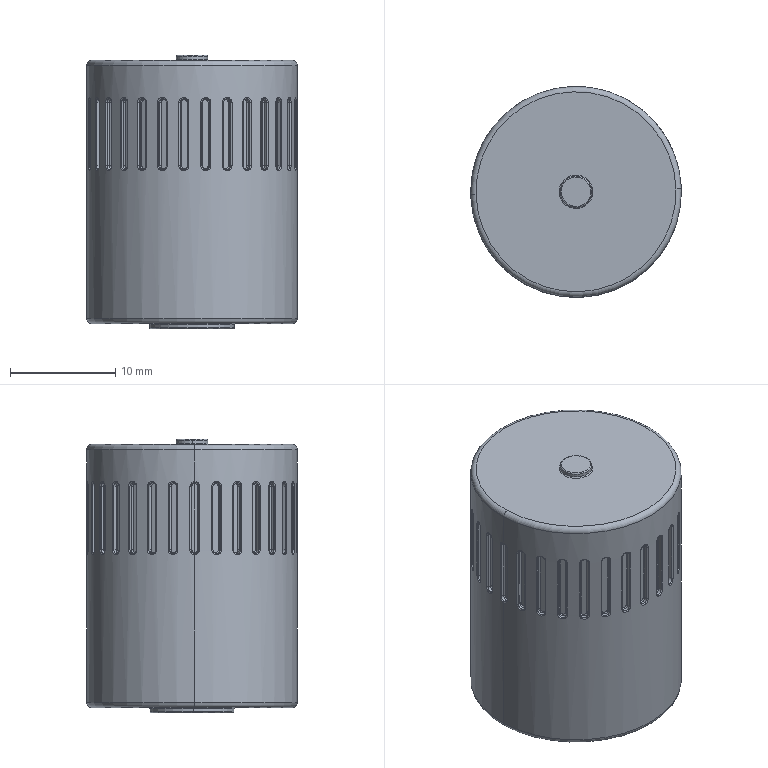Part | SolidWorks | features SplitBody 1 | 1 solid | 474 faces | box 20 x 20 x 26 mm | volume 7738 mm3 | cylinder 261 | spline 120 | plane 69 | torus 24 | commonest cylinder face diameters 0.2 x152 0.75 x62 20 x33 1.25 x6 3 x4 5 x2